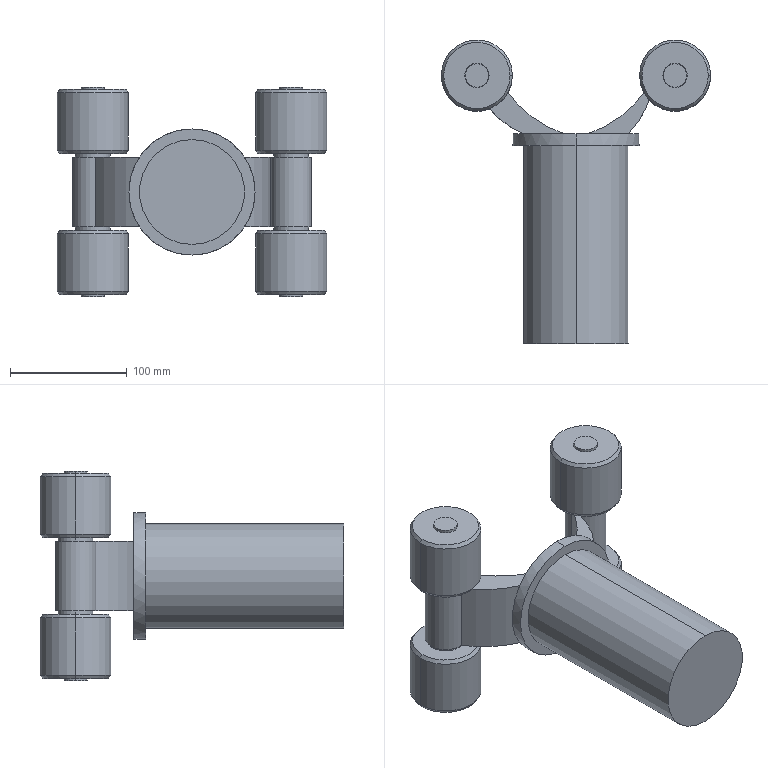Part | SolidWorks | features ICE 5, MirrorPattern 2, Extrusion 1, RefAxis 1, Revolution 1 | 1 solid | 84 faces | box 231 x 260.5 x 180 mm | volume 2038334 mm3 | cylinder 43 | plane 25 | cone 16 | commonest cylinder face diameters 20 x8 21 x8 30 x8 61 x8 35 x3 90 x2